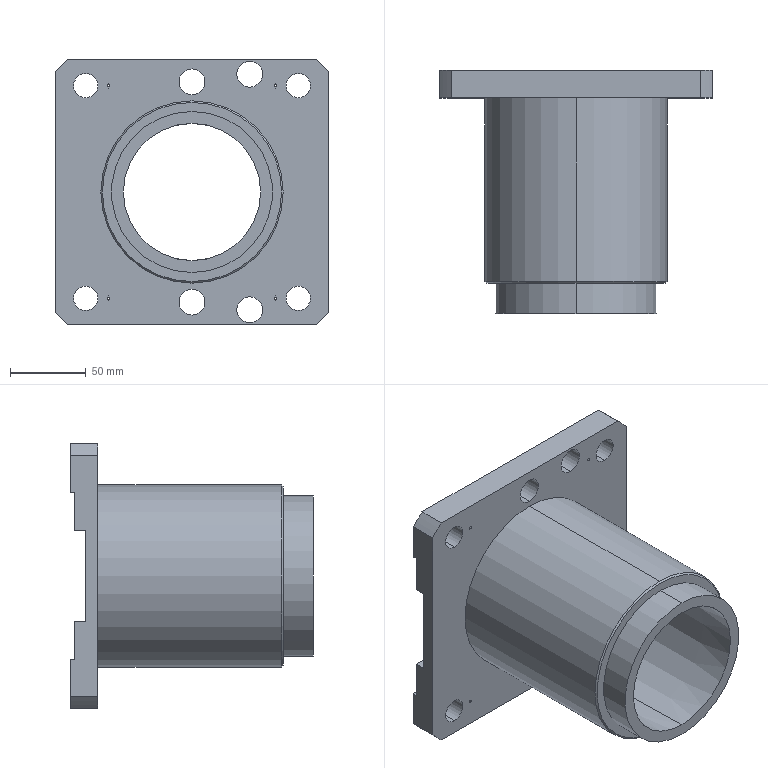Part | STEP file | PN_0016 Snap-ring guide sleeve | 1 solid | 72 faces | box 180 x 160 x 175 mm | volume 921190 mm3 | cylinder 35 | plane 19 | cone 18 | commonest cylinder face diameters 5 x8 16 x8 17 x8 240 x4 97.4 x3 106 x2